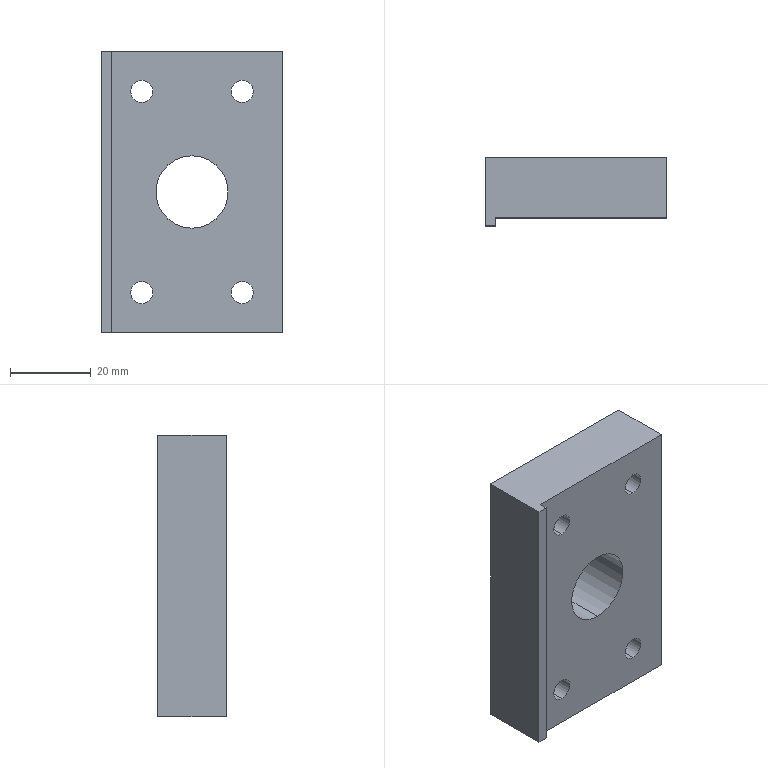Part | SolidWorks | features HoleWzd 3, Cut 1, Extrusion 1 | 1 solid | 38 faces | box 45 x 17 x 70 mm | volume 40738 mm3 | cylinder 22 | plane 12 | cone 4 | commonest cylinder face diameters 5.5 x8 10 x8 2.5 x4 18 x2
STEP:
#1=CARTESIAN_POINT('',(14.,-1.5,-6.25));
#2=VERTEX_POINT('',#1);
#3=CARTESIAN_POINT('',(14.,-1.5,-8.75));
#4=VERTEX_POINT('',#3);
#5=CARTESIAN_POINT('',(14.,-1.5,-7.5));
#6=DIRECTION('',(1.,0.,0.));
#7=DIRECTION('',(0.,0.,-1.));
#8=AXIS2_PLACEMENT_3D('',#5,#6,#7);
#9=CIRCLE('',#8,1.25);
#10=EDGE_CURVE('',#2,#4,#9,.T.);
#11=ORIENTED_EDGE('',*,*,#10,.F.);
#12=CARTESIAN_POINT('',(22.5,-1.5,-6.25));
#13=VERTEX_POINT('',#12);
#14=CARTESIAN_POINT('',(22.5,-1.5,-6.25));
#15=DIRECTION('',(1.,0.,0.));
#16=VECTOR('',#15,1000.);
#17=LINE('',#14,#16);
#18=EDGE_CURVE('',#2,#13,#17,.T.);
#19=ORIENTED_EDGE('',*,*,#18,.T.);
#20=CARTESIAN_POINT('',(22.5,-1.5,-8.75));
#21=VERTEX_POINT('',#20);
#22=CARTESIAN_POINT('',(22.5,-1.5,-7.5));
#23=DIRECTION('',(1.,0.,0.));
#24=DIRECTION('',(0.,0.,-1.));
#25=AXIS2_PLACEMENT_3D('',#22,#23,#24);
#26=CIRCLE('',#25,1.25);
#27=EDGE_CURVE('',#13,#21,#26,.T.);
#28=ORIENTED_EDGE('',*,*,#27,.T.);
#29=CARTESIAN_POINT('',(22.5,-1.5,-8.75));
#30=DIRECTION('',(1.,0.,0.));
#31=VECTOR('',#30,1000.);
#32=LINE('',#29,#31);
#33=EDGE_CURVE('',#4,#21,#32,.T.);
#34=ORIENTED_EDGE('',*,*,#33,.F.);
#35=EDGE_LOOP('',(#11,#19,#28,#34));
#36=FACE_OUTER_BOUND('',#35,.T.);
#37=CARTESIAN_POINT('',(22.5,-1.5,-7.5));
#38=DIRECTION('',(1.,0.,0.));
#39=DIRECTION('',(0.,0.,-1.));
#40=AXIS2_PLACEMENT_3D('',#37,#38,#39);
#41=CYLINDRICAL_SURFACE('',#40,1.25);
#42=ADVANCED_FACE('',(#36),#41,.F.);
#43=CARTESIAN_POINT('',(13.249,-1.5,-7.5));
#44=VERTEX_POINT('',#43);
#45=CARTESIAN_POINT('',(14.,-1.5,-8.75));
#46=DIRECTION('',(0.515,0.,-0.8572));
#47=VECTOR('',#46,1000.);
#48=LINE('',#45,#47);
#49=EDGE_CURVE('',#44,#4,#48,.T.);
#50=ORIENTED_EDGE('',*,*,#49,.F.);
#51=CARTESIAN_POINT('',(14.,-1.5,-6.25));
#52=DIRECTION('',(0.515,0.,0.8572));
#53=VECTOR('',#52,1000.);
#54=LINE('',#51,#53);
#55=EDGE_CURVE('',#44,#2,#54,.T.);
#56=ORIENTED_EDGE('',*,*,#55,.T.);
#57=ORIENTED_EDGE('',*,*,#10,.T.);
#58=EDGE_LOOP('',(#50,#56,#57));
#59=FACE_OUTER_BOUND('',#58,.T.);
#60=CARTESIAN_POINT('',(14.,-1.5,-7.5));
#61=DIRECTION('',(1.,0.,0.));
#62=DIRECTION('',(0.,0.,-1.));
#63=AXIS2_PLACEMENT_3D('',#60,#61,#62);
#64=CONICAL_SURFACE('',#63,1.25,1.03);
#65=ADVANCED_FACE('',(#59),#64,.F.);
#66=CARTESIAN_POINT('',(14.,-1.5,8.75));
#67=VERTEX_POINT('',#66);
#68=CARTESIAN_POINT('',(14.,-1.5,6.25));
#69=VERTEX_POINT('',#68);
#70=CARTESIAN_POINT('',(14.,-1.5,7.5));
#71=DIRECTION('',(1.,0.,0.));
#72=DIRECTION('',(0.,0.,-1.));
#73=AXIS2_PLACEMENT_3D('',#70,#71,#72);
#74=CIRCLE('',#73,1.25);
#75=EDGE_CURVE('',#67,#69,#74,.T.);
#76=ORIENTED_EDGE('',*,*,#75,.F.);
#77=CARTESIAN_POINT('',(22.5,-1.5,8.75));
#78=VERTEX_POINT('',#77);
#79=CARTESIAN_POINT('',(22.5,-1.5,8.75));
#80=DIRECTION('',(1.,0.,0.));
#81=VECTOR('',#80,1000.);
#82=LINE('',#79,#81);
#83=EDGE_CURVE('',#67,#78,#82,.T.);
#84=ORIENTED_EDGE('',*,*,#83,.T.);
#85=CARTESIAN_POINT('',(22.5,-1.5,6.25));
#86=VERTEX_POINT('',#85);
#87=CARTESIAN_POINT('',(22.5,-1.5,7.5));
#88=DIRECTION('',(1.,0.,0.));
#89=DIRECTION('',(0.,0.,-1.));
#90=AXIS2_PLACEMENT_3D('',#87,#88,#89);
#91=CIRCLE('',#90,1.25);
#92=EDGE_CURVE('',#78,#86,#91,.T.);
#93=ORIENTED_EDGE('',*,*,#92,.T.);
#94=CARTESIAN_POINT('',(22.5,-1.5,6.25));
#95=DIRECTION('',(1.,0.,0.));
#96=VECTOR('',#95,1000.);
#97=LINE('',#94,#96);
#98=EDGE_CURVE('',#69,#86,#97,.T.);
#99=ORIENTED_EDGE('',*,*,#98,.F.);
#100=EDGE_LOOP('',(#76,#84,#93,#99));
#101=FACE_OUTER_BOUND('',#100,.T.);
#102=CARTESIAN_POINT('',(22.5,-1.5,7.5));
#103=DIRECTION('',(1.,0.,0.));
#104=DIRECTION('',(0.,0.,-1.));
#105=AXIS2_PLACEMENT_3D('',#102,#103,#104);
#106=CYLINDRICAL_SURFACE('',#105,1.25);
#107=ADVANCED_FACE('',(#101),#106,.F.);
#108=CARTESIAN_POINT('',(13.249,-1.5,7.5));
#109=VERTEX_POINT('',#108);
#110=CARTESIAN_POINT('',(14.,-1.5,6.25));
#111=DIRECTION('',(0.515,0.,-0.8572));
#112=VECTOR('',#111,1000.);
#113=LINE('',#110,#112);
#114=EDGE_CURVE('',#109,#69,#113,.T.);
#115=ORIENTED_EDGE('',*,*,#114,.F.);
#116=CARTESIAN_POINT('',(14.,-1.5,8.75));
#117=DIRECTION('',(0.515,0.,0.8572));
#118=VECTOR('',#117,1000.);
#119=LINE('',#116,#118);
#120=EDGE_CURVE('',#109,#67,#119,.T.);
#121=ORIENTED_EDGE('',*,*,#120,.T.);
#122=ORIENTED_EDGE('',*,*,#75,.T.);
#123=EDGE_LOOP('',(#115,#121,#122));
#124=FACE_OUTER_BOUND('',#123,.T.);
#125=CARTESIAN_POINT('',(14.,-1.5,7.5));
#126=DIRECTION('',(1.,0.,0.));
#127=DIRECTION('',(0.,0.,-1.));
#128=AXIS2_PLACEMENT_3D('',#125,#126,#127);
#129=CONICAL_SURFACE('',#128,1.25,1.03);
#130=ADVANCED_FACE('',(#124),#129,.F.);
#131=CARTESIAN_POINT('',(0.,-6.5,9.));
#132=VERTEX_POINT('',#131);
#133=CARTESIAN_POINT('',(0.,-6.5,-9.));
#134=VERTEX_POINT('',#133);
#135=CARTESIAN_POINT('',(0.,-6.5,0.));
#136=DIRECTION('',(0.,-1.,0.));
#137=DIRECTION('',(0.,0.,-1.));
#138=AXIS2_PLACEMENT_3D('',#135,#136,#137);
#139=CIRCLE('',#138,9.);
#140=EDGE_CURVE('',#132,#134,#139,.T.);
#141=ORIENTED_EDGE('',*,*,#140,.T.);
#142=CARTESIAN_POINT('',(0.,8.5,-9.));
#143=VERTEX_POINT('',#142);
#144=CARTESIAN_POINT('',(0.,8.5,-9.));
#145=DIRECTION('',(0.,1.,0.));
#146=VECTOR('',#145,1000.);
#147=LINE('',#144,#146);
#148=EDGE_CURVE('',#134,#143,#147,.T.);
#149=ORIENTED_EDGE('',*,*,#148,.T.);
#150=CARTESIAN_POINT('',(0.,8.5,9.));
#151=VERTEX_POINT('',#150);
#152=CARTESIAN_POINT('',(0.,8.5,0.));
#153=DIRECTION('',(0.,1.,0.));
#154=DIRECTION('',(0.,0.,1.));
#155=AXIS2_PLACEMENT_3D('',#152,#153,#154);
#156=CIRCLE('',#155,9.);
#157=EDGE_CURVE('',#143,#151,#156,.T.);
#158=ORIENTED_EDGE('',*,*,#157,.T.);
#159=CARTESIAN_POINT('',(0.,8.5,9.));
#160=DIRECTION('',(0.,1.,0.));
#161=VECTOR('',#160,1000.);
#162=LINE('',#159,#161);
#163=EDGE_CURVE('',#132,#151,#162,.T.);
#164=ORIENTED_EDGE('',*,*,#163,.F.);
#165=EDGE_LOOP('',(#141,#149,#158,#164));
#166=FACE_OUTER_BOUND('',#165,.T.);
#167=CARTESIAN_POINT('',(0.,8.5,0.));
#168=DIRECTION('',(0.,1.,0.));
#169=DIRECTION('',(0.,0.,1.));
#170=AXIS2_PLACEMENT_3D('',#167,#168,#169);
#171=CYLINDRICAL_SURFACE('',#170,9.);
#172=ADVANCED_FACE('',(#166),#171,.F.);
#173=CARTESIAN_POINT('',(-12.5,1.5,20.));
#174=VERTEX_POINT('',#173);
#175=CARTESIAN_POINT('',(-12.5,1.5,30.));
#176=VERTEX_POINT('',#175);
#177=CARTESIAN_POINT('',(-12.5,1.5,25.));
#178=DIRECTION('',(0.,1.,0.));
#179=DIRECTION('',(0.,0.,1.));
#180=AXIS2_PLACEMENT_3D('',#177,#178,#179);
#181=CIRCLE('',#180,5.);
#182=EDGE_CURVE('',#174,#176,#181,.T.);
#183=ORIENTED_EDGE('',*,*,#182,.F.);
#184=CARTESIAN_POINT('',(-12.5,8.5,20.));
#185=VERTEX_POINT('',#184);
#186=CARTESIAN_POINT('',(-12.5,8.5,20.));
#187=DIRECTION('',(0.,1.,0.));
#188=VECTOR('',#187,1000.);
#189=LINE('',#186,#188);
#190=EDGE_CURVE('',#174,#185,#189,.T.);
#191=ORIENTED_EDGE('',*,*,#190,.T.);
#192=CARTESIAN_POINT('',(-12.5,8.5,30.));
#193=VERTEX_POINT('',#192);
#194=CARTESIAN_POINT('',(-12.5,8.5,25.));
#195=DIRECTION('',(0.,1.,0.));
#196=DIRECTION('',(0.,0.,1.));
#197=AXIS2_PLACEMENT_3D('',#194,#195,#196);
#198=CIRCLE('',#197,5.);
#199=EDGE_CURVE('',#185,#193,#198,.T.);
#200=ORIENTED_EDGE('',*,*,#199,.T.);
#201=CARTESIAN_POINT('',(-12.5,8.5,30.));
#202=DIRECTION('',(0.,1.,0.));
#203=VECTOR('',#202,1000.);
#204=LINE('',#201,#203);
#205=EDGE_CURVE('',#176,#193,#204,.T.);
#206=ORIENTED_EDGE('',*,*,#205,.F.);
#207=EDGE_LOOP('',(#183,#191,#200,#206));
#208=FACE_OUTER_BOUND('',#207,.T.);
#209=CARTESIAN_POINT('',(-12.5,8.5,25.));
#210=DIRECTION('',(0.,1.,0.));
#211=DIRECTION('',(0.,0.,1.));
#212=AXIS2_PLACEMENT_3D('',#209,#210,#211);
#213=CYLINDRICAL_SURFACE('',#212,5.);
#214=ADVANCED_FACE('',(#208),#213,.F.);
#215=CARTESIAN_POINT('',(-12.5,-6.5,27.75));
#216=VERTEX_POINT('',#215);
#217=CARTESIAN_POINT('',(-12.5,-6.5,22.25));
#218=VERTEX_POINT('',#217);
#219=CARTESIAN_POINT('',(-12.5,-6.5,25.));
#220=DIRECTION('',(0.,-1.,0.));
#221=DIRECTION('',(0.,0.,-1.));
#222=AXIS2_PLACEMENT_3D('',#219,#220,#221);
#223=CIRCLE('',#222,2.75);
#224=EDGE_CURVE('',#216,#218,#223,.T.);
#225=ORIENTED_EDGE('',*,*,#224,.T.);
#226=CARTESIAN_POINT('',(-12.5,1.5,22.25));
#227=VERTEX_POINT('',#226);
#228=CARTESIAN_POINT('',(-12.5,8.5,22.25));
#229=DIRECTION('',(0.,1.,0.));
#230=VECTOR('',#229,1000.);
#231=LINE('',#228,#230);
#232=EDGE_CURVE('',#218,#227,#231,.T.);
#233=ORIENTED_EDGE('',*,*,#232,.T.);
#234=CARTESIAN_POINT('',(-12.5,1.5,27.75));
#235=VERTEX_POINT('',#234);
#236=CARTESIAN_POINT('',(-12.5,1.5,25.));
#237=DIRECTION('',(0.,1.,0.));
#238=DIRECTION('',(0.,0.,1.));
#239=AXIS2_PLACEMENT_3D('',#236,#237,#238);
#240=CIRCLE('',#239,2.75);
#241=EDGE_CURVE('',#227,#235,#240,.T.);
#242=ORIENTED_EDGE('',*,*,#241,.T.);
#243=CARTESIAN_POINT('',(-12.5,8.5,27.75));
#244=DIRECTION('',(0.,1.,0.));
#245=VECTOR('',#244,1000.);
#246=LINE('',#243,#245);
#247=EDGE_CURVE('',#216,#235,#246,.T.);
#248=ORIENTED_EDGE('',*,*,#247,.F.);
#249=EDGE_LOOP('',(#225,#233,#242,#248));
#250=FACE_OUTER_BOUND('',#249,.T.);
#251=CARTESIAN_POINT('',(-12.5,8.5,25.));
#252=DIRECTION('',(0.,1.,0.));
#253=DIRECTION('',(0.,0.,1.));
#254=AXIS2_PLACEMENT_3D('',#251,#252,#253);
#255=CYLINDRICAL_SURFACE('',#254,2.75);
#256=ADVANCED_FACE('',(#250),#255,.F.);
#257=CARTESIAN_POINT('',(-12.5,1.5,-30.));
#258=VERTEX_POINT('',#257);
#259=CARTESIAN_POINT('',(-12.5,1.5,-20.));
#260=VERTEX_POINT('',#259);
#261=CARTESIAN_POINT('',(-12.5,1.5,-25.));
#262=DIRECTION('',(0.,1.,0.));
#263=DIRECTION('',(0.,0.,1.));
#264=AXIS2_PLACEMENT_3D('',#261,#262,#263);
#265=CIRCLE('',#264,5.);
#266=EDGE_CURVE('',#258,#260,#265,.T.);
#267=ORIENTED_EDGE('',*,*,#266,.F.);
#268=CARTESIAN_POINT('',(-12.5,8.5,-30.));
#269=VERTEX_POINT('',#268);
#270=CARTESIAN_POINT('',(-12.5,8.5,-30.));
#271=DIRECTION('',(0.,1.,0.));
#272=VECTOR('',#271,1000.);
#273=LINE('',#270,#272);
#274=EDGE_CURVE('',#258,#269,#273,.T.);
#275=ORIENTED_EDGE('',*,*,#274,.T.);
#276=CARTESIAN_POINT('',(-12.5,8.5,-20.));
#277=VERTEX_POINT('',#276);
#278=CARTESIAN_POINT('',(-12.5,8.5,-25.));
#279=DIRECTION('',(0.,1.,0.));
#280=DIRECTION('',(0.,0.,1.));
#281=AXIS2_PLACEMENT_3D('',#278,#279,#280);
#282=CIRCLE('',#281,5.);
#283=EDGE_CURVE('',#269,#277,#282,.T.);
#284=ORIENTED_EDGE('',*,*,#283,.T.);
#285=CARTESIAN_POINT('',(-12.5,8.5,-20.));
#286=DIRECTION('',(0.,1.,0.));
#287=VECTOR('',#286,1000.);
#288=LINE('',#285,#287);
#289=EDGE_CURVE('',#260,#277,#288,.T.);
#290=ORIENTED_EDGE('',*,*,#289,.F.);
#291=EDGE_LOOP('',(#267,#275,#284,#290));
#292=FACE_OUTER_BOUND('',#291,.T.);
#293=CARTESIAN_POINT('',(-12.5,8.5,-25.));
#294=DIRECTION('',(0.,1.,0.));
#295=DIRECTION('',(0.,0.,1.));
#296=AXIS2_PLACEMENT_3D('',#293,#294,#295);
#297=CYLINDRICAL_SURFACE('',#296,5.);
#298=ADVANCED_FACE('',(#292),#297,.F.);
#299=CARTESIAN_POINT('',(-12.5,-6.5,-22.25));
#300=VERTEX_POINT('',#299);
#301=CARTESIAN_POINT('',(-12.5,-6.5,-27.75));
#302=VERTEX_POINT('',#301);
#303=CARTESIAN_POINT('',(-12.5,-6.5,-25.));
#304=DIRECTION('',(0.,-1.,0.));
#305=DIRECTION('',(0.,0.,-1.));
#306=AXIS2_PLACEMENT_3D('',#303,#304,#305);
#307=CIRCLE('',#306,2.75);
#308=EDGE_CURVE('',#300,#302,#307,.T.);
#309=ORIENTED_EDGE('',*,*,#308,.T.);
#310=CARTESIAN_POINT('',(-12.5,1.5,-27.75));
#311=VERTEX_POINT('',#310);
#312=CARTESIAN_POINT('',(-12.5,8.5,-27.75));
#313=DIRECTION('',(0.,1.,0.));
#314=VECTOR('',#313,1000.);
#315=LINE('',#312,#314);
#316=EDGE_CURVE('',#302,#311,#315,.T.);
#317=ORIENTED_EDGE('',*,*,#316,.T.);
#318=CARTESIAN_POINT('',(-12.5,1.5,-22.25));
#319=VERTEX_POINT('',#318);
#320=CARTESIAN_POINT('',(-12.5,1.5,-25.));
#321=DIRECTION('',(0.,1.,0.));
#322=DIRECTION('',(0.,0.,1.));
#323=AXIS2_PLACEMENT_3D('',#320,#321,#322);
#324=CIRCLE('',#323,2.75);
#325=EDGE_CURVE('',#311,#319,#324,.T.);
#326=ORIENTED_EDGE('',*,*,#325,.T.);
#327=CARTESIAN_POINT('',(-12.5,8.5,-22.25));
#328=DIRECTION('',(0.,1.,0.));
#329=VECTOR('',#328,1000.);
#330=LINE('',#327,#329);
#331=EDGE_CURVE('',#300,#319,#330,.T.);
#332=ORIENTED_EDGE('',*,*,#331,.F.);
#333=EDGE_LOOP('',(#309,#317,#326,#332));
#334=FACE_OUTER_BOUND('',#333,.T.);
#335=CARTESIAN_POINT('',(-12.5,8.5,-25.));
#336=DIRECTION('',(0.,1.,0.));
#337=DIRECTION('',(0.,0.,1.));
#338=AXIS2_PLACEMENT_3D('',#335,#336,#337);
#339=CYLINDRICAL_SURFACE('',#338,2.75);
#340=ADVANCED_FACE('',(#334),#339,.F.);
#341=CARTESIAN_POINT('',(12.5,1.5,-30.));
#342=VERTEX_POINT('',#341);
#343=CARTESIAN_POINT('',(12.5,1.5,-20.));
#344=VERTEX_POINT('',#343);
#345=CARTESIAN_POINT('',(12.5,1.5,-25.));
#346=DIRECTION('',(0.,1.,0.));
#347=DIRECTION('',(0.,0.,1.));
#348=AXIS2_PLACEMENT_3D('',#345,#346,#347);
#349=CIRCLE('',#348,5.);
#350=EDGE_CURVE('',#342,#344,#349,.T.);
#351=ORIENTED_EDGE('',*,*,#350,.F.);
#352=CARTESIAN_POINT('',(12.5,8.5,-30.));
#353=VERTEX_POINT('',#352);
#354=CARTESIAN_POINT('',(12.5,8.5,-30.));
#355=DIRECTION('',(0.,1.,0.));
#356=VECTOR('',#355,1000.);
#357=LINE('',#354,#356);
#358=EDGE_CURVE('',#342,#353,#357,.T.);
#359=ORIENTED_EDGE('',*,*,#358,.T.);
#360=CARTESIAN_POINT('',(12.5,8.5,-20.));
#361=VERTEX_POINT('',#360);
#362=CARTESIAN_POINT('',(12.5,8.5,-25.));
#363=DIRECTION('',(0.,1.,0.));
#364=DIRECTION('',(0.,0.,1.));
#365=AXIS2_PLACEMENT_3D('',#362,#363,#364);
#366=CIRCLE('',#365,5.);
#367=EDGE_CURVE('',#353,#361,#366,.T.);
#368=ORIENTED_EDGE('',*,*,#367,.T.);
#369=CARTESIAN_POINT('',(12.5,8.5,-20.));
#370=DIRECTION('',(0.,1.,0.));
#371=VECTOR('',#370,1000.);
#372=LINE('',#369,#371);
#373=EDGE_CURVE('',#344,#361,#372,.T.);
#374=ORIENTED_EDGE('',*,*,#373,.F.);
#375=EDGE_LOOP('',(#351,#359,#368,#374));
#376=FACE_OUTER_BOUND('',#375,.T.);
#377=CARTESIAN_POINT('',(12.5,8.5,-25.));
#378=DIRECTION('',(0.,1.,0.));
#379=DIRECTION('',(0.,0.,1.));
#380=AXIS2_PLACEMENT_3D('',#377,#378,#379);
#381=CYLINDRICAL_SURFACE('',#380,5.);
#382=ADVANCED_FACE('',(#376),#381,.F.);
#383=CARTESIAN_POINT('',(12.5,-6.5,-22.25));
#384=VERTEX_POINT('',#383);
#385=CARTESIAN_POINT('',(12.5,-6.5,-27.75));
#386=VERTEX_POINT('',#385);
#387=CARTESIAN_POINT('',(12.5,-6.5,-25.));
#388=DIRECTION('',(0.,-1.,0.));
#389=DIRECTION('',(0.,0.,-1.));
#390=AXIS2_PLACEMENT_3D('',#387,#388,#389);
#391=CIRCLE('',#390,2.75);
#392=EDGE_CURVE('',#384,#386,#391,.T.);
#393=ORIENTED_EDGE('',*,*,#392,.T.);
#394=CARTESIAN_POINT('',(12.5,1.5,-27.75));
#395=VERTEX_POINT('',#394);
#396=CARTESIAN_POINT('',(12.5,8.5,-27.75));
#397=DIRECTION('',(0.,1.,0.));
#398=VECTOR('',#397,1000.);
#399=LINE('',#396,#398);
#400=EDGE_CURVE('',#386,#395,#399,.T.);
#401=ORIENTED_EDGE('',*,*,#400,.T.);
#402=CARTESIAN_POINT('',(12.5,1.5,-22.25));
#403=VERTEX_POINT('',#402);
#404=CARTESIAN_POINT('',(12.5,1.5,-25.));
#405=DIRECTION('',(0.,1.,0.));
#406=DIRECTION('',(0.,0.,1.));
#407=AXIS2_PLACEMENT_3D('',#404,#405,#406);
#408=CIRCLE('',#407,2.75);
#409=EDGE_CURVE('',#395,#403,#408,.T.);
#410=ORIENTED_EDGE('',*,*,#409,.T.);
#411=CARTESIAN_POINT('',(12.5,8.5,-22.25));
#412=DIRECTION('',(0.,1.,0.));
#413=VECTOR('',#412,1000.);
#414=LINE('',#411,#413);
#415=EDGE_CURVE('',#384,#403,#414,.T.);
#416=ORIENTED_EDGE('',*,*,#415,.F.);
#417=EDGE_LOOP('',(#393,#401,#410,#416));
#418=FACE_OUTER_BOUND('',#417,.T.);
#419=CARTESIAN_POINT('',(12.5,8.5,-25.));
#420=DIRECTION('',(0.,1.,0.));
#421=DIRECTION('',(0.,0.,1.));
#422=AXIS2_PLACEMENT_3D('',#419,#420,#421);
#423=CYLINDRICAL_SURFACE('',#422,2.75);
#424=ADVANCED_FACE('',(#418),#423,.F.);
#425=CARTESIAN_POINT('',(12.5,1.5,20.));
#426=VERTEX_POINT('',#425);
#427=CARTESIAN_POINT('',(12.5,1.5,30.));
#428=VERTEX_POINT('',#427);
#429=CARTESIAN_POINT('',(12.5,1.5,25.));
#430=DIRECTION('',(0.,1.,0.));
#431=DIRECTION('',(0.,0.,1.));
#432=AXIS2_PLACEMENT_3D('',#429,#430,#431);
#433=CIRCLE('',#432,5.);
#434=EDGE_CURVE('',#426,#428,#433,.T.);
#435=ORIENTED_EDGE('',*,*,#434,.F.);
#436=CARTESIAN_POINT('',(12.5,8.5,20.));
#437=VERTEX_POINT('',#436);
#438=CARTESIAN_POINT('',(12.5,8.5,20.));
#439=DIRECTION('',(0.,1.,0.));
#440=VECTOR('',#439,1000.);
#441=LINE('',#438,#440);
#442=EDGE_CURVE('',#426,#437,#441,.T.);
#443=ORIENTED_EDGE('',*,*,#442,.T.);
#444=CARTESIAN_POINT('',(12.5,8.5,30.));
#445=VERTEX_POINT('',#444);
#446=CARTESIAN_POINT('',(12.5,8.5,25.));
#447=DIRECTION('',(0.,1.,0.));
#448=DIRECTION('',(0.,0.,1.));
#449=AXIS2_PLACEMENT_3D('',#446,#447,#448);
#450=CIRCLE('',#449,5.);
#451=EDGE_CURVE('',#437,#445,#450,.T.);
#452=ORIENTED_EDGE('',*,*,#451,.T.);
#453=CARTESIAN_POINT('',(12.5,8.5,30.));
#454=DIRECTION('',(0.,1.,0.));
#455=VECTOR('',#454,1000.);
#456=LINE('',#453,#455);
#457=EDGE_CURVE('',#428,#445,#456,.T.);
#458=ORIENTED_EDGE('',*,*,#457,.F.);
#459=EDGE_LOOP('',(#435,#443,#452,#458));
#460=FACE_OUTER_BOUND('',#459,.T.);
#461=CARTESIAN_POINT('',(12.5,8.5,25.));
#462=DIRECTION('',(0.,1.,0.));
#463=DIRECTION('',(0.,0.,1.));
#464=AXIS2_PLACEMENT_3D('',#461,#462,#463);
#465=CYLINDRICAL_SURFACE('',#464,5.);
#466=ADVANCED_FACE('',(#460),#465,.F.);
#467=CARTESIAN_POINT('',(12.5,-6.5,27.75));
#468=VERTEX_POINT('',#467);
#469=CARTESIAN_POINT('',(12.5,-6.5,22.25));
#470=VERTEX_POINT('',#469);
#471=CARTESIAN_POINT('',(12.5,-6.5,25.));
#472=DIRECTION('',(0.,-1.,0.));
#473=DIRECTION('',(0.,0.,-1.));
#474=AXIS2_PLACEMENT_3D('',#471,#472,#473);
#475=CIRCLE('',#474,2.75);
#476=EDGE_CURVE('',#468,#470,#475,.T.);
#477=ORIENTED_EDGE('',*,*,#476,.T.);
#478=CARTESIAN_POINT('',(12.5,1.5,22.25));
#479=VERTEX_POINT('',#478);
#480=CARTESIAN_POINT('',(12.5,8.5,22.25));
#481=DIRECTION('',(0.,1.,0.));
#482=VECTOR('',#481,1000.);
#483=LINE('',#480,#482);
#484=EDGE_CURVE('',#470,#479,#483,.T.);
#485=ORIENTED_EDGE('',*,*,#484,.T.);
#486=CARTESIAN_POINT('',(12.5,1.5,27.75));
#487=VERTEX_POINT('',#486);
#488=CARTESIAN_POINT('',(12.5,1.5,25.));
#489=DIRECTION('',(0.,1.,0.));
#490=DIRECTION('',(0.,0.,1.));
#491=AXIS2_PLACEMENT_3D('',#488,#489,#490);
#492=CIRCLE('',#491,2.75);
#493=EDGE_CURVE('',#479,#487,#492,.T.);
#494=ORIENTED_EDGE('',*,*,#493,.T.);
#495=CARTESIAN_POINT('',(12.5,8.5,27.75));
#496=DIRECTION('',(0.,1.,0.));
#497=VECTOR('',#496,1000.);
#498=LINE('',#495,#497);
#499=EDGE_CURVE('',#468,#487,#498,.T.);
#500=ORIENTED_EDGE('',*,*,#499,.F.);
#501=EDGE_LOOP('',(#477,#485,#494,#500));
#502=FACE_OUTER_BOUND('',#501,.T.);
#503=CARTESIAN_POINT('',(12.5,8.5,25.));
#504=DIRECTION('',(0.,1.,0.));
#505=DIRECTION('',(0.,0.,1.));
#506=AXIS2_PLACEMENT_3D('',#503,#504,#505);
#507=CYLINDRICAL_SURFACE('',#506,2.75);
#508=ADVANCED_FACE('',(#502),#507,.F.);
#509=CARTESIAN_POINT('',(22.5,-1.5,-7.5));
#510=DIRECTION('',(1.,0.,0.));
#511=DIRECTION('',(0.,0.,-1.));
#512=AXIS2_PLACEMENT_3D('',#509,#510,#511);
#513=CIRCLE('',#512,1.25);
#514=EDGE_CURVE('',#21,#13,#513,.T.);
#515=ORIENTED_EDGE('',*,*,#514,.F.);
#516=ORIENTED_EDGE('',*,*,#27,.F.);
#517=EDGE_LOOP('',(#515,#516));
#518=FACE_BOUND('',#517,.T.);
#519=CARTESIAN_POINT('',(22.5,-1.5,7.5));
#520=DIRECTION('',(1.,0.,0.));
#521=DIRECTION('',(0.,0.,-1.));
#522=AXIS2_PLACEMENT_3D('',#519,#520,#521);
#523=CIRCLE('',#522,1.25);
#524=EDGE_CURVE('',#86,#78,#523,.T.);
#525=ORIENTED_EDGE('',*,*,#524,.F.);
#526=ORIENTED_EDGE('',*,*,#92,.F.);
#527=EDGE_LOOP('',(#525,#526));
#528=FACE_BOUND('',#527,.T.);
#529=CARTESIAN_POINT('',(22.5,-6.5,-35.));
#530=VERTEX_POINT('',#529);
#531=CARTESIAN_POINT('',(22.5,-6.5,35.));
#532=VERTEX_POINT('',#531);
#533=CARTESIAN_POINT('',(22.5,-6.5,35.));
#534=DIRECTION('',(0.,0.,1.));
#535=VECTOR('',#534,1000.);
#536=LINE('',#533,#535);
#537=EDGE_CURVE('',#530,#532,#536,.T.);
#538=ORIENTED_EDGE('',*,*,#537,.F.);
#539=CARTESIAN_POINT('',(22.5,8.5,-35.));
#540=VERTEX_POINT('',#539);
#541=CARTESIAN_POINT('',(22.5,8.5,-35.));
#542=DIRECTION('',(0.,-1.,0.));
#543=VECTOR('',#542,1000.);
#544=LINE('',#541,#543);
#545=EDGE_CURVE('',#540,#530,#544,.T.);
#546=ORIENTED_EDGE('',*,*,#545,.F.);
#547=CARTESIAN_POINT('',(22.5,8.5,35.));
#548=VERTEX_POINT('',#547);
#549=CARTESIAN_POINT('',(22.5,8.5,35.));
#550=DIRECTION('',(0.,0.,-1.));
#551=VECTOR('',#550,1000.);
#552=LINE('',#549,#551);
#553=EDGE_CURVE('',#548,#540,#552,.T.);
#554=ORIENTED_EDGE('',*,*,#553,.F.);
#555=CARTESIAN_POINT('',(22.5,8.5,35.));
#556=DIRECTION('',(0.,-1.,0.));
#557=VECTOR('',#556,1000.);
#558=LINE('',#555,#557);
#559=EDGE_CURVE('',#548,#532,#558,.T.);
#560=ORIENTED_EDGE('',*,*,#559,.T.);
#561=EDGE_LOOP('',(#538,#546,#554,#560));
#562=FACE_OUTER_BOUND('',#561,.T.);
#563=CARTESIAN_POINT('',(22.5,8.5,35.));
#564=DIRECTION('',(-1.,0.,0.));
#565=DIRECTION('',(0.,0.,1.));
#566=AXIS2_PLACEMENT_3D('',#563,#564,#565);
#567=PLANE('',#566);
#568=ADVANCED_FACE('',(#518,#528,#562),#567,.F.);
#569=CARTESIAN_POINT('',(-22.5,-8.5,-35.));
#570=VERTEX_POINT('',#569);
#571=CARTESIAN_POINT('',(-22.5,-8.5,35.));
#572=VERTEX_POINT('',#571);
#573=CARTESIAN_POINT('',(-22.5,-8.5,35.));
#574=DIRECTION('',(0.,0.,1.));
#575=VECTOR('',#574,1000.);
#576=LINE('',#573,#575);
#577=EDGE_CURVE('',#570,#572,#576,.T.);
#578=ORIENTED_EDGE('',*,*,#577,.T.);
#579=CARTESIAN_POINT('',(-22.5,8.5,35.));
#580=VERTEX_POINT('',#579);
#581=CARTESIAN_POINT('',(-22.5,8.5,35.));
#582=DIRECTION('',(0.,-1.,0.));
#583=VECTOR('',#582,1000.);
#584=LINE('',#581,#583);
#585=EDGE_CURVE('',#580,#572,#584,.T.);
#586=ORIENTED_EDGE('',*,*,#585,.F.);
#587=CARTESIAN_POINT('',(-22.5,8.5,-35.));
#588=VERTEX_POINT('',#587);
#589=CARTESIAN_POINT('',(-22.5,8.5,35.));
#590=DIRECTION('',(0.,0.,1.));
#591=VECTOR('',#590,1000.);
#592=LINE('',#589,#591);
#593=EDGE_CURVE('',#588,#580,#592,.T.);
#594=ORIENTED_EDGE('',*,*,#593,.F.);
#595=CARTESIAN_POINT('',(-22.5,8.5,-35.));
#596=DIRECTION('',(0.,-1.,0.));
#597=VECTOR('',#596,1000.);
#598=LINE('',#595,#597);
#599=EDGE_CURVE('',#588,#570,#598,.T.);
#600=ORIENTED_EDGE('',*,*,#599,.T.);
#601=EDGE_LOOP('',(#578,#586,#594,#600));
#602=FACE_OUTER_BOUND('',#601,.T.);
#603=CARTESIAN_POINT('',(-22.5,8.5,35.));
#604=DIRECTION('',(1.,0.,0.));
#605=DIRECTION('',(0.,0.,-1.));
#606=AXIS2_PLACEMENT_3D('',#603,#604,#605);
#607=PLANE('',#606);
#608=ADVANCED_FACE('',(#602),#607,.F.);
#609=CARTESIAN_POINT('',(-20.,-8.5,35.));
#610=VERTEX_POINT('',#609);
#611=CARTESIAN_POINT('',(22.5,-8.5,35.));
#612=DIRECTION('',(1.,0.,0.));
#613=VECTOR('',#612,1000.);
#614=LINE('',#611,#613);
#615=EDGE_CURVE('',#572,#610,#614,.T.);
#616=ORIENTED_EDGE('',*,*,#615,.T.);
#617=CARTESIAN_POINT('',(-20.,-6.5,35.));
#618=VERTEX_POINT('',#617);
#619=CARTESIAN_POINT('',(-20.,-6.5,35.));
#620=DIRECTION('',(0.,-1.,0.));
#621=VECTOR('',#620,1000.);
#622=LINE('',#619,#621);
#623=EDGE_CURVE('',#618,#610,#622,.T.);
#624=ORIENTED_EDGE('',*,*,#623,.F.);
#625=CARTESIAN_POINT('',(-20.,-6.5,35.));
#626=DIRECTION('',(-1.,0.,0.));
#627=VECTOR('',#626,1000.);
#628=LINE('',#625,#627);
#629=EDGE_CURVE('',#532,#618,#628,.T.);
#630=ORIENTED_EDGE('',*,*,#629,.F.);
#631=ORIENTED_EDGE('',*,*,#559,.F.);
#632=CARTESIAN_POINT('',(22.5,8.5,35.));
#633=DIRECTION('',(1.,0.,0.));
#634=VECTOR('',#633,1000.);
#635=LINE('',#632,#634);
#636=EDGE_CURVE('',#580,#548,#635,.T.);
#637=ORIENTED_EDGE('',*,*,#636,.F.);
#638=ORIENTED_EDGE('',*,*,#585,.T.);
#639=EDGE_LOOP('',(#616,#624,#630,#631,#637,#638));
#640=FACE_OUTER_BOUND('',#639,.T.);
#641=CARTESIAN_POINT('',(22.5,8.5,35.));
#642=DIRECTION('',(0.,0.,-1.));
#643=DIRECTION('',(-1.,0.,0.));
#644=AXIS2_PLACEMENT_3D('',#641,#642,#643);
#645=PLANE('',#644);
#646=ADVANCED_FACE('',(#640),#645,.F.);
#647=CARTESIAN_POINT('',(-20.,-6.5,-35.));
#648=VERTEX_POINT('',#647);
#649=CARTESIAN_POINT('',(-20.,-6.5,-35.));
#650=DIRECTION('',(1.,0.,0.));
#651=VECTOR('',#650,1000.);
#652=LINE('',#649,#651);
#653=EDGE_CURVE('',#648,#530,#652,.T.);
#654=ORIENTED_EDGE('',*,*,#653,.F.);
#655=CARTESIAN_POINT('',(-20.,-8.5,-35.));
#656=VERTEX_POINT('',#655);
#657=CARTESIAN_POINT('',(-20.,-6.5,-35.));
#658=DIRECTION('',(0.,-1.,0.));
#659=VECTOR('',#658,1000.);
#660=LINE('',#657,#659);
#661=EDGE_CURVE('',#648,#656,#660,.T.);
#662=ORIENTED_EDGE('',*,*,#661,.T.);
#663=CARTESIAN_POINT('',(22.5,-8.5,-35.));
#664=DIRECTION('',(-1.,0.,0.));
#665=VECTOR('',#664,1000.);
#666=LINE('',#663,#665);
#667=EDGE_CURVE('',#656,#570,#666,.T.);
#668=ORIENTED_EDGE('',*,*,#667,.T.);
#669=ORIENTED_EDGE('',*,*,#599,.F.);
#670=CARTESIAN_POINT('',(22.5,8.5,-35.));
#671=DIRECTION('',(-1.,0.,0.));
#672=VECTOR('',#671,1000.);
#673=LINE('',#670,#672);
#674=EDGE_CURVE('',#540,#588,#673,.T.);
#675=ORIENTED_EDGE('',*,*,#674,.F.);
#676=ORIENTED_EDGE('',*,*,#545,.T.);
#677=EDGE_LOOP('',(#654,#662,#668,#669,#675,#676));
#678=FACE_OUTER_BOUND('',#677,.T.);
#679=CARTESIAN_POINT('',(22.5,8.5,-35.));
#680=DIRECTION('',(0.,0.,1.));
#681=DIRECTION('',(1.,0.,0.));
#682=AXIS2_PLACEMENT_3D('',#679,#680,#681);
#683=PLANE('',#682);
#684=ADVANCED_FACE('',(#678),#683,.F.);
#685=CARTESIAN_POINT('',(0.,8.5,0.));
#686=DIRECTION('',(0.,1.,0.));
#687=DIRECTION('',(0.,0.,1.));
#688=AXIS2_PLACEMENT_3D('',#685,#686,#687);
#689=CIRCLE('',#688,9.);
#690=EDGE_CURVE('',#151,#143,#689,.T.);
#691=ORIENTED_EDGE('',*,*,#690,.F.);
#692=ORIENTED_EDGE('',*,*,#157,.F.);
#693=EDGE_LOOP('',(#691,#692));
#694=FACE_BOUND('',#693,.T.);
#695=CARTESIAN_POINT('',(-12.5,8.5,25.));
#696=DIRECTION('',(0.,1.,0.));
#697=DIRECTION('',(0.,0.,1.));
#698=AXIS2_PLACEMENT_3D('',#695,#696,#697);
#699=CIRCLE('',#698,5.);
#700=EDGE_CURVE('',#193,#185,#699,.T.);
#701=ORIENTED_EDGE('',*,*,#700,.F.);
#702=ORIENTED_EDGE('',*,*,#199,.F.);
#703=EDGE_LOOP('',(#701,#702));
#704=FACE_BOUND('',#703,.T.);
#705=CARTESIAN_POINT('',(-12.5,8.5,-25.));
#706=DIRECTION('',(0.,1.,0.));
#707=DIRECTION('',(0.,0.,1.));
#708=AXIS2_PLACEMENT_3D('',#705,#706,#707);
#709=CIRCLE('',#708,5.);
#710=EDGE_CURVE('',#277,#269,#709,.T.);
#711=ORIENTED_EDGE('',*,*,#710,.F.);
#712=ORIENTED_EDGE('',*,*,#283,.F.);
#713=EDGE_LOOP('',(#711,#712));
#714=FACE_BOUND('',#713,.T.);
#715=CARTESIAN_POINT('',(12.5,8.5,-25.));
#716=DIRECTION('',(0.,1.,0.));
#717=DIRECTION('',(0.,0.,1.));
#718=AXIS2_PLACEMENT_3D('',#715,#716,#717);
#719=CIRCLE('',#718,5.);
#720=EDGE_CURVE('',#361,#353,#719,.T.);
#721=ORIENTED_EDGE('',*,*,#720,.F.);
#722=ORIENTED_EDGE('',*,*,#367,.F.);
#723=EDGE_LOOP('',(#721,#722));
#724=FACE_BOUND('',#723,.T.);
#725=CARTESIAN_POINT('',(12.5,8.5,25.));
#726=DIRECTION('',(0.,1.,0.));
#727=DIRECTION('',(0.,0.,1.));
#728=AXIS2_PLACEMENT_3D('',#725,#726,#727);
#729=CIRCLE('',#728,5.);
#730=EDGE_CURVE('',#445,#437,#729,.T.);
#731=ORIENTED_EDGE('',*,*,#730,.F.);
#732=ORIENTED_EDGE('',*,*,#451,.F.);
#733=EDGE_LOOP('',(#731,#732));
#734=FACE_BOUND('',#733,.T.);
#735=ORIENTED_EDGE('',*,*,#593,.T.);
#736=ORIENTED_EDGE('',*,*,#636,.T.);
#737=ORIENTED_EDGE('',*,*,#553,.T.);
#738=ORIENTED_EDGE('',*,*,#674,.T.);
#739=EDGE_LOOP('',(#735,#736,#737,#738));
#740=FACE_OUTER_BOUND('',#739,.T.);
#741=CARTESIAN_POINT('',(0.,8.5,0.));
#742=DIRECTION('',(0.,1.,0.));
#743=DIRECTION('',(0.,0.,1.));
#744=AXIS2_PLACEMENT_3D('',#741,#742,#743);
#745=PLANE('',#744);
#746=ADVANCED_FACE('',(#694,#704,#714,#724,#734,#740),#745,.T.);
#747=ORIENTED_EDGE('',*,*,#667,.F.);
#748=CARTESIAN_POINT('',(-20.,-8.5,35.));
#749=DIRECTION('',(0.,0.,-1.));
#750=VECTOR('',#749,1000.);
#751=LINE('',#748,#750);
#752=EDGE_CURVE('',#610,#656,#751,.T.);
#753=ORIENTED_EDGE('',*,*,#752,.F.);
#754=ORIENTED_EDGE('',*,*,#615,.F.);
#755=ORIENTED_EDGE('',*,*,#577,.F.);
#756=EDGE_LOOP('',(#747,#753,#754,#755));
#757=FACE_OUTER_BOUND('',#756,.T.);
#758=CARTESIAN_POINT('',(0.,-8.5,0.));
#759=DIRECTION('',(0.,1.,0.));
#760=DIRECTION('',(0.,0.,1.));
#761=AXIS2_PLACEMENT_3D('',#758,#759,#760);
#762=PLANE('',#761);
#763=ADVANCED_FACE('',(#757),#762,.F.);
#764=ORIENTED_EDGE('',*,*,#752,.T.);
#765=ORIENTED_EDGE('',*,*,#661,.F.);
#766=CARTESIAN_POINT('',(-20.,-6.5,35.));
#767=DIRECTION('',(0.,0.,-1.));
#768=VECTOR('',#767,1000.);
#769=LINE('',#766,#768);
#770=EDGE_CURVE('',#618,#648,#769,.T.);
#771=ORIENTED_EDGE('',*,*,#770,.F.);
#772=ORIENTED_EDGE('',*,*,#623,.T.);
#773=EDGE_LOOP('',(#764,#765,#771,#772));
#774=FACE_OUTER_BOUND('',#773,.T.);
#775=CARTESIAN_POINT('',(-20.,-6.5,35.));
#776=DIRECTION('',(-1.,0.,0.));
#777=DIRECTION('',(0.,0.,1.));
#778=AXIS2_PLACEMENT_3D('',#775,#776,#777);
#779=PLANE('',#778);
#780=ADVANCED_FACE('',(#774),#779,.F.);
#781=ORIENTED_EDGE('',*,*,#140,.F.);
#782=CARTESIAN_POINT('',(0.,-6.5,0.));
#783=DIRECTION('',(0.,-1.,0.));
#784=DIRECTION('',(0.,0.,-1.));
#785=AXIS2_PLACEMENT_3D('',#782,#783,#784);
#786=CIRCLE('',#785,9.);
#787=EDGE_CURVE('',#134,#132,#786,.T.);
#788=ORIENTED_EDGE('',*,*,#787,.F.);
#789=EDGE_LOOP('',(#781,#788));
#790=FACE_BOUND('',#789,.T.);
#791=ORIENTED_EDGE('',*,*,#224,.F.);
#792=CARTESIAN_POINT('',(-12.5,-6.5,25.));
#793=DIRECTION('',(0.,-1.,0.));
#794=DIRECTION('',(0.,0.,-1.));
#795=AXIS2_PLACEMENT_3D('',#792,#793,#794);
#796=CIRCLE('',#795,2.75);
#797=EDGE_CURVE('',#218,#216,#796,.T.);
#798=ORIENTED_EDGE('',*,*,#797,.F.);
#799=EDGE_LOOP('',(#791,#798));
#800=FACE_BOUND('',#799,.T.);
#801=ORIENTED_EDGE('',*,*,#308,.F.);
#802=CARTESIAN_POINT('',(-12.5,-6.5,-25.));
#803=DIRECTION('',(0.,-1.,0.));
#804=DIRECTION('',(0.,0.,-1.));
#805=AXIS2_PLACEMENT_3D('',#802,#803,#804);
#806=CIRCLE('',#805,2.75);
#807=EDGE_CURVE('',#302,#300,#806,.T.);
#808=ORIENTED_EDGE('',*,*,#807,.F.);
#809=EDGE_LOOP('',(#801,#808));
#810=FACE_BOUND('',#809,.T.);
#811=ORIENTED_EDGE('',*,*,#392,.F.);
#812=CARTESIAN_POINT('',(12.5,-6.5,-25.));
#813=DIRECTION('',(0.,-1.,0.));
#814=DIRECTION('',(0.,0.,-1.));
#815=AXIS2_PLACEMENT_3D('',#812,#813,#814);
#816=CIRCLE('',#815,2.75);
#817=EDGE_CURVE('',#386,#384,#816,.T.);
#818=ORIENTED_EDGE('',*,*,#817,.F.);
#819=EDGE_LOOP('',(#811,#818));
#820=FACE_BOUND('',#819,.T.);
#821=ORIENTED_EDGE('',*,*,#476,.F.);
#822=CARTESIAN_POINT('',(12.5,-6.5,25.));
#823=DIRECTION('',(0.,-1.,0.));
#824=DIRECTION('',(0.,0.,-1.));
#825=AXIS2_PLACEMENT_3D('',#822,#823,#824);
#826=CIRCLE('',#825,2.75);
#827=EDGE_CURVE('',#470,#468,#826,.T.);
#828=ORIENTED_EDGE('',*,*,#827,.F.);
#829=EDGE_LOOP('',(#821,#828));
#830=FACE_BOUND('',#829,.T.);
#831=ORIENTED_EDGE('',*,*,#770,.T.);
#832=ORIENTED_EDGE('',*,*,#653,.T.);
#833=ORIENTED_EDGE('',*,*,#537,.T.);
#834=ORIENTED_EDGE('',*,*,#629,.T.);
#835=EDGE_LOOP('',(#831,#832,#833,#834));
#836=FACE_OUTER_BOUND('',#835,.T.);
#837=CARTESIAN_POINT('',(0.,-6.5,0.));
#838=DIRECTION('',(0.,-1.,0.));
#839=DIRECTION('',(0.,0.,-1.));
#840=AXIS2_PLACEMENT_3D('',#837,#838,#839);
#841=PLANE('',#840);
#842=ADVANCED_FACE('',(#790,#800,#810,#820,#830,#836),#841,.T.);
#843=ORIENTED_EDGE('',*,*,#484,.F.);
#844=ORIENTED_EDGE('',*,*,#827,.T.);
#845=ORIENTED_EDGE('',*,*,#499,.T.);
#846=CARTESIAN_POINT('',(12.5,1.5,25.));
#847=DIRECTION('',(0.,1.,0.));
#848=DIRECTION('',(0.,0.,1.));
#849=AXIS2_PLACEMENT_3D('',#846,#847,#848);
#850=CIRCLE('',#849,2.75);
#851=EDGE_CURVE('',#487,#479,#850,.T.);
#852=ORIENTED_EDGE('',*,*,#851,.T.);
#853=EDGE_LOOP('',(#843,#844,#845,#852));
#854=FACE_OUTER_BOUND('',#853,.T.);
#855=CARTESIAN_POINT('',(12.5,8.5,25.));
#856=DIRECTION('',(0.,1.,0.));
#857=DIRECTION('',(0.,0.,1.));
#858=AXIS2_PLACEMENT_3D('',#855,#856,#857);
#859=CYLINDRICAL_SURFACE('',#858,2.75);
#860=ADVANCED_FACE('',(#854),#859,.F.);
#861=ORIENTED_EDGE('',*,*,#851,.F.);
#862=ORIENTED_EDGE('',*,*,#493,.F.);
#863=EDGE_LOOP('',(#861,#862));
#864=FACE_BOUND('',#863,.T.);
#865=CARTESIAN_POINT('',(12.5,1.5,25.));
#866=DIRECTION('',(0.,1.,0.));
#867=DIRECTION('',(0.,0.,1.));
#868=AXIS2_PLACEMENT_3D('',#865,#866,#867);
#869=CIRCLE('',#868,5.);
#870=EDGE_CURVE('',#428,#426,#869,.T.);
#871=ORIENTED_EDGE('',*,*,#870,.T.);
#872=ORIENTED_EDGE('',*,*,#434,.T.);
#873=EDGE_LOOP('',(#871,#872));
#874=FACE_OUTER_BOUND('',#873,.T.);
#875=CARTESIAN_POINT('',(15.25,1.5,25.));
#876=DIRECTION('',(0.,-1.,0.));
#877=DIRECTION('',(0.,0.,-1.));
#878=AXIS2_PLACEMENT_3D('',#875,#876,#877);
#879=PLANE('',#878);
#880=ADVANCED_FACE('',(#864,#874),#879,.F.);
#881=ORIENTED_EDGE('',*,*,#442,.F.);
#882=ORIENTED_EDGE('',*,*,#870,.F.);
#883=ORIENTED_EDGE('',*,*,#457,.T.);
#884=ORIENTED_EDGE('',*,*,#730,.T.);
#885=EDGE_LOOP('',(#881,#882,#883,#884));
#886=FACE_OUTER_BOUND('',#885,.T.);
#887=CARTESIAN_POINT('',(12.5,8.5,25.));
#888=DIRECTION('',(0.,1.,0.));
#889=DIRECTION('',(0.,0.,1.));
#890=AXIS2_PLACEMENT_3D('',#887,#888,#889);
#891=CYLINDRICAL_SURFACE('',#890,5.);
#892=ADVANCED_FACE('',(#886),#891,.F.);
#893=ORIENTED_EDGE('',*,*,#400,.F.);
#894=ORIENTED_EDGE('',*,*,#817,.T.);
#895=ORIENTED_EDGE('',*,*,#415,.T.);
#896=CARTESIAN_POINT('',(12.5,1.5,-25.));
#897=DIRECTION('',(0.,1.,0.));
#898=DIRECTION('',(0.,0.,1.));
#899=AXIS2_PLACEMENT_3D('',#896,#897,#898);
#900=CIRCLE('',#899,2.75);
#901=EDGE_CURVE('',#403,#395,#900,.T.);
#902=ORIENTED_EDGE('',*,*,#901,.T.);
#903=EDGE_LOOP('',(#893,#894,#895,#902));
#904=FACE_OUTER_BOUND('',#903,.T.);
#905=CARTESIAN_POINT('',(12.5,8.5,-25.));
#906=DIRECTION('',(0.,1.,0.));
#907=DIRECTION('',(0.,0.,1.));
#908=AXIS2_PLACEMENT_3D('',#905,#906,#907);
#909=CYLINDRICAL_SURFACE('',#908,2.75);
#910=ADVANCED_FACE('',(#904),#909,.F.);
#911=ORIENTED_EDGE('',*,*,#901,.F.);
#912=ORIENTED_EDGE('',*,*,#409,.F.);
#913=EDGE_LOOP('',(#911,#912));
#914=FACE_BOUND('',#913,.T.);
#915=CARTESIAN_POINT('',(12.5,1.5,-25.));
#916=DIRECTION('',(0.,1.,0.));
#917=DIRECTION('',(0.,0.,1.));
#918=AXIS2_PLACEMENT_3D('',#915,#916,#917);
#919=CIRCLE('',#918,5.);
#920=EDGE_CURVE('',#344,#342,#919,.T.);
#921=ORIENTED_EDGE('',*,*,#920,.T.);
#922=ORIENTED_EDGE('',*,*,#350,.T.);
#923=EDGE_LOOP('',(#921,#922));
#924=FACE_OUTER_BOUND('',#923,.T.);
#925=CARTESIAN_POINT('',(15.25,1.5,-25.));
#926=DIRECTION('',(0.,-1.,0.));
#927=DIRECTION('',(0.,0.,-1.));
#928=AXIS2_PLACEMENT_3D('',#925,#926,#927);
#929=PLANE('',#928);
#930=ADVANCED_FACE('',(#914,#924),#929,.F.);
#931=ORIENTED_EDGE('',*,*,#358,.F.);
#932=ORIENTED_EDGE('',*,*,#920,.F.);
#933=ORIENTED_EDGE('',*,*,#373,.T.);
#934=ORIENTED_EDGE('',*,*,#720,.T.);
#935=EDGE_LOOP('',(#931,#932,#933,#934));
#936=FACE_OUTER_BOUND('',#935,.T.);
#937=CARTESIAN_POINT('',(12.5,8.5,-25.));
#938=DIRECTION('',(0.,1.,0.));
#939=DIRECTION('',(0.,0.,1.));
#940=AXIS2_PLACEMENT_3D('',#937,#938,#939);
#941=CYLINDRICAL_SURFACE('',#940,5.);
#942=ADVANCED_FACE('',(#936),#941,.F.);
#943=ORIENTED_EDGE('',*,*,#316,.F.);
#944=ORIENTED_EDGE('',*,*,#807,.T.);
#945=ORIENTED_EDGE('',*,*,#331,.T.);
#946=CARTESIAN_POINT('',(-12.5,1.5,-25.));
#947=DIRECTION('',(0.,1.,0.));
#948=DIRECTION('',(0.,0.,1.));
#949=AXIS2_PLACEMENT_3D('',#946,#947,#948);
#950=CIRCLE('',#949,2.75);
#951=EDGE_CURVE('',#319,#311,#950,.T.);
#952=ORIENTED_EDGE('',*,*,#951,.T.);
#953=EDGE_LOOP('',(#943,#944,#945,#952));
#954=FACE_OUTER_BOUND('',#953,.T.);
#955=CARTESIAN_POINT('',(-12.5,8.5,-25.));
#956=DIRECTION('',(0.,1.,0.));
#957=DIRECTION('',(0.,0.,1.));
#958=AXIS2_PLACEMENT_3D('',#955,#956,#957);
#959=CYLINDRICAL_SURFACE('',#958,2.75);
#960=ADVANCED_FACE('',(#954),#959,.F.);
#961=ORIENTED_EDGE('',*,*,#951,.F.);
#962=ORIENTED_EDGE('',*,*,#325,.F.);
#963=EDGE_LOOP('',(#961,#962));
#964=FACE_BOUND('',#963,.T.);
#965=CARTESIAN_POINT('',(-12.5,1.5,-25.));
#966=DIRECTION('',(0.,1.,0.));
#967=DIRECTION('',(0.,0.,1.));
#968=AXIS2_PLACEMENT_3D('',#965,#966,#967);
#969=CIRCLE('',#968,5.);
#970=EDGE_CURVE('',#260,#258,#969,.T.);
#971=ORIENTED_EDGE('',*,*,#970,.T.);
#972=ORIENTED_EDGE('',*,*,#266,.T.);
#973=EDGE_LOOP('',(#971,#972));
#974=FACE_OUTER_BOUND('',#973,.T.);
#975=CARTESIAN_POINT('',(-9.75,1.5,-25.));
#976=DIRECTION('',(0.,-1.,0.));
#977=DIRECTION('',(0.,0.,-1.));
#978=AXIS2_PLACEMENT_3D('',#975,#976,#977);
#979=PLANE('',#978);
#980=ADVANCED_FACE('',(#964,#974),#979,.F.);
#981=ORIENTED_EDGE('',*,*,#274,.F.);
#982=ORIENTED_EDGE('',*,*,#970,.F.);
#983=ORIENTED_EDGE('',*,*,#289,.T.);
#984=ORIENTED_EDGE('',*,*,#710,.T.);
#985=EDGE_LOOP('',(#981,#982,#983,#984));
#986=FACE_OUTER_BOUND('',#985,.T.);
#987=CARTESIAN_POINT('',(-12.5,8.5,-25.));
#988=DIRECTION('',(0.,1.,0.));
#989=DIRECTION('',(0.,0.,1.));
#990=AXIS2_PLACEMENT_3D('',#987,#988,#989);
#991=CYLINDRICAL_SURFACE('',#990,5.);
#992=ADVANCED_FACE('',(#986),#991,.F.);
#993=ORIENTED_EDGE('',*,*,#232,.F.);
#994=ORIENTED_EDGE('',*,*,#797,.T.);
#995=ORIENTED_EDGE('',*,*,#247,.T.);
#996=CARTESIAN_POINT('',(-12.5,1.5,25.));
#997=DIRECTION('',(0.,1.,0.));
#998=DIRECTION('',(0.,0.,1.));
#999=AXIS2_PLACEMENT_3D('',#996,#997,#998);
#1000=CIRCLE('',#999,2.75);
#1001=EDGE_CURVE('',#235,#227,#1000,.T.);
#1002=ORIENTED_EDGE('',*,*,#1001,.T.);
#1003=EDGE_LOOP('',(#993,#994,#995,#1002));
#1004=FACE_OUTER_BOUND('',#1003,.T.);
#1005=CARTESIAN_POINT('',(-12.5,8.5,25.));
#1006=DIRECTION('',(0.,1.,0.));
#1007=DIRECTION('',(0.,0.,1.));
#1008=AXIS2_PLACEMENT_3D('',#1005,#1006,#1007);
#1009=CYLINDRICAL_SURFACE('',#1008,2.75);
#1010=ADVANCED_FACE('',(#1004),#1009,.F.);
#1011=ORIENTED_EDGE('',*,*,#1001,.F.);
#1012=ORIENTED_EDGE('',*,*,#241,.F.);
#1013=EDGE_LOOP('',(#1011,#1012));
#1014=FACE_BOUND('',#1013,.T.);
#1015=CARTESIAN_POINT('',(-12.5,1.5,25.));
#1016=DIRECTION('',(0.,1.,0.));
#1017=DIRECTION('',(0.,0.,1.));
#1018=AXIS2_PLACEMENT_3D('',#1015,#1016,#1017);
#1019=CIRCLE('',#1018,5.);
#1020=EDGE_CURVE('',#176,#174,#1019,.T.);
#1021=ORIENTED_EDGE('',*,*,#1020,.T.);
#1022=ORIENTED_EDGE('',*,*,#182,.T.);
#1023=EDGE_LOOP('',(#1021,#1022));
#1024=FACE_OUTER_BOUND('',#1023,.T.);
#1025=CARTESIAN_POINT('',(-9.75,1.5,25.));
#1026=DIRECTION('',(0.,-1.,0.));
#1027=DIRECTION('',(0.,0.,-1.));
#1028=AXIS2_PLACEMENT_3D('',#1025,#1026,#1027);
#1029=PLANE('',#1028);
#1030=ADVANCED_FACE('',(#1014,#1024),#1029,.F.);
#1031=ORIENTED_EDGE('',*,*,#190,.F.);
#1032=ORIENTED_EDGE('',*,*,#1020,.F.);
#1033=ORIENTED_EDGE('',*,*,#205,.T.);
#1034=ORIENTED_EDGE('',*,*,#700,.T.);
#1035=EDGE_LOOP('',(#1031,#1032,#1033,#1034));
#1036=FACE_OUTER_BOUND('',#1035,.T.);
#1037=CARTESIAN_POINT('',(-12.5,8.5,25.));
#1038=DIRECTION('',(0.,1.,0.));
#1039=DIRECTION('',(0.,0.,1.));
#1040=AXIS2_PLACEMENT_3D('',#1037,#1038,#1039);
#1041=CYLINDRICAL_SURFACE('',#1040,5.);
#1042=ADVANCED_FACE('',(#1036),#1041,.F.);
#1043=ORIENTED_EDGE('',*,*,#148,.F.);
#1044=ORIENTED_EDGE('',*,*,#787,.T.);
#1045=ORIENTED_EDGE('',*,*,#163,.T.);
#1046=ORIENTED_EDGE('',*,*,#690,.T.);
#1047=EDGE_LOOP('',(#1043,#1044,#1045,#1046));
#1048=FACE_OUTER_BOUND('',#1047,.T.);
#1049=CARTESIAN_POINT('',(0.,8.5,0.));
#1050=DIRECTION('',(0.,1.,0.));
#1051=DIRECTION('',(0.,0.,1.));
#1052=AXIS2_PLACEMENT_3D('',#1049,#1050,#1051);
#1053=CYLINDRICAL_SURFACE('',#1052,9.);
#1054=ADVANCED_FACE('',(#1048),#1053,.F.);
#1055=ORIENTED_EDGE('',*,*,#120,.F.);
#1056=ORIENTED_EDGE('',*,*,#114,.T.);
#1057=CARTESIAN_POINT('',(14.,-1.5,7.5));
#1058=DIRECTION('',(1.,0.,0.));
#1059=DIRECTION('',(0.,0.,-1.));
#1060=AXIS2_PLACEMENT_3D('',#1057,#1058,#1059);
#1061=CIRCLE('',#1060,1.25);
#1062=EDGE_CURVE('',#69,#67,#1061,.T.);
#1063=ORIENTED_EDGE('',*,*,#1062,.T.);
#1064=EDGE_LOOP('',(#1055,#1056,#1063));
#1065=FACE_OUTER_BOUND('',#1064,.T.);
#1066=CARTESIAN_POINT('',(14.,-1.5,7.5));
#1067=DIRECTION('',(1.,0.,0.));
#1068=DIRECTION('',(0.,0.,-1.));
#1069=AXIS2_PLACEMENT_3D('',#1066,#1067,#1068);
#1070=CONICAL_SURFACE('',#1069,1.25,1.03);
#1071=ADVANCED_FACE('',(#1065),#1070,.F.);
#1072=ORIENTED_EDGE('',*,*,#83,.F.);
#1073=ORIENTED_EDGE('',*,*,#1062,.F.);
#1074=ORIENTED_EDGE('',*,*,#98,.T.);
#1075=ORIENTED_EDGE('',*,*,#524,.T.);
#1076=EDGE_LOOP('',(#1072,#1073,#1074,#1075));
#1077=FACE_OUTER_BOUND('',#1076,.T.);
#1078=CARTESIAN_POINT('',(22.5,-1.5,7.5));
#1079=DIRECTION('',(1.,0.,0.));
#1080=DIRECTION('',(0.,0.,-1.));
#1081=AXIS2_PLACEMENT_3D('',#1078,#1079,#1080);
#1082=CYLINDRICAL_SURFACE('',#1081,1.25);
#1083=ADVANCED_FACE('',(#1077),#1082,.F.);
#1084=ORIENTED_EDGE('',*,*,#55,.F.);
#1085=ORIENTED_EDGE('',*,*,#49,.T.);
#1086=CARTESIAN_POINT('',(14.,-1.5,-7.5));
#1087=DIRECTION('',(1.,0.,0.));
#1088=DIRECTION('',(0.,0.,-1.));
#1089=AXIS2_PLACEMENT_3D('',#1086,#1087,#1088);
#1090=CIRCLE('',#1089,1.25);
#1091=EDGE_CURVE('',#4,#2,#1090,.T.);
#1092=ORIENTED_EDGE('',*,*,#1091,.T.);
#1093=EDGE_LOOP('',(#1084,#1085,#1092));
#1094=FACE_OUTER_BOUND('',#1093,.T.);
#1095=CARTESIAN_POINT('',(14.,-1.5,-7.5));
#1096=DIRECTION('',(1.,0.,0.));
#1097=DIRECTION('',(0.,0.,-1.));
#1098=AXIS2_PLACEMENT_3D('',#1095,#1096,#1097);
#1099=CONICAL_SURFACE('',#1098,1.25,1.03);
#1100=ADVANCED_FACE('',(#1094),#1099,.F.);
#1101=ORIENTED_EDGE('',*,*,#18,.F.);
#1102=ORIENTED_EDGE('',*,*,#1091,.F.);
#1103=ORIENTED_EDGE('',*,*,#33,.T.);
#1104=ORIENTED_EDGE('',*,*,#514,.T.);
#1105=EDGE_LOOP('',(#1101,#1102,#1103,#1104));
#1106=FACE_OUTER_BOUND('',#1105,.T.);
#1107=CARTESIAN_POINT('',(22.5,-1.5,-7.5));
#1108=DIRECTION('',(1.,0.,0.));
#1109=DIRECTION('',(0.,0.,-1.));
#1110=AXIS2_PLACEMENT_3D('',#1107,#1108,#1109);
#1111=CYLINDRICAL_SURFACE('',#1110,1.25);
#1112=ADVANCED_FACE('',(#1106),#1111,.F.);
#1113=CLOSED_SHELL('',(#42,#65,#107,#130,#172,#214,#256,#298,#340,#382,#424,#466,#508,#568,#608,#646,#684,#746,#763,#780,#842,#860,#880,#892,#910,#930,#942,#960,#980,#992,#1010,#1030,#1042,#1054,#1071,#1083,#1100,#1112));
#1114=MANIFOLD_SOLID_BREP('',#1113);
#1115=CARTESIAN_POINT('',(0.,0.,0.));
#1116=DIRECTION('',(0.,0.,1.));
#1117=DIRECTION('',(1.,0.,0.));
#1118=AXIS2_PLACEMENT_3D('',#1115,#1116,#1117);
#1119=(LENGTH_UNIT()NAMED_UNIT(*)SI_UNIT(.MILLI.,.METRE.));
#1120=UNCERTAINTY_MEASURE_WITH_UNIT(LENGTH_MEASURE(0.00001),#1119,'','');
#1121=(NAMED_UNIT(*)PLANE_ANGLE_UNIT()SI_UNIT($,.RADIAN.));
#1122=(NAMED_UNIT(*)SI_UNIT($,.STERADIAN.)SOLID_ANGLE_UNIT());
#1123=(GEOMETRIC_REPRESENTATION_CONTEXT(3)GLOBAL_UNCERTAINTY_ASSIGNED_CONTEXT((#1120))GLOBAL_UNIT_ASSIGNED_CONTEXT((#1119,#1121,#1122))REPRESENTATION_CONTEXT('',''));
#1124=ADVANCED_BREP_SHAPE_REPRESENTATION('',(#1114,#1118),#1123);